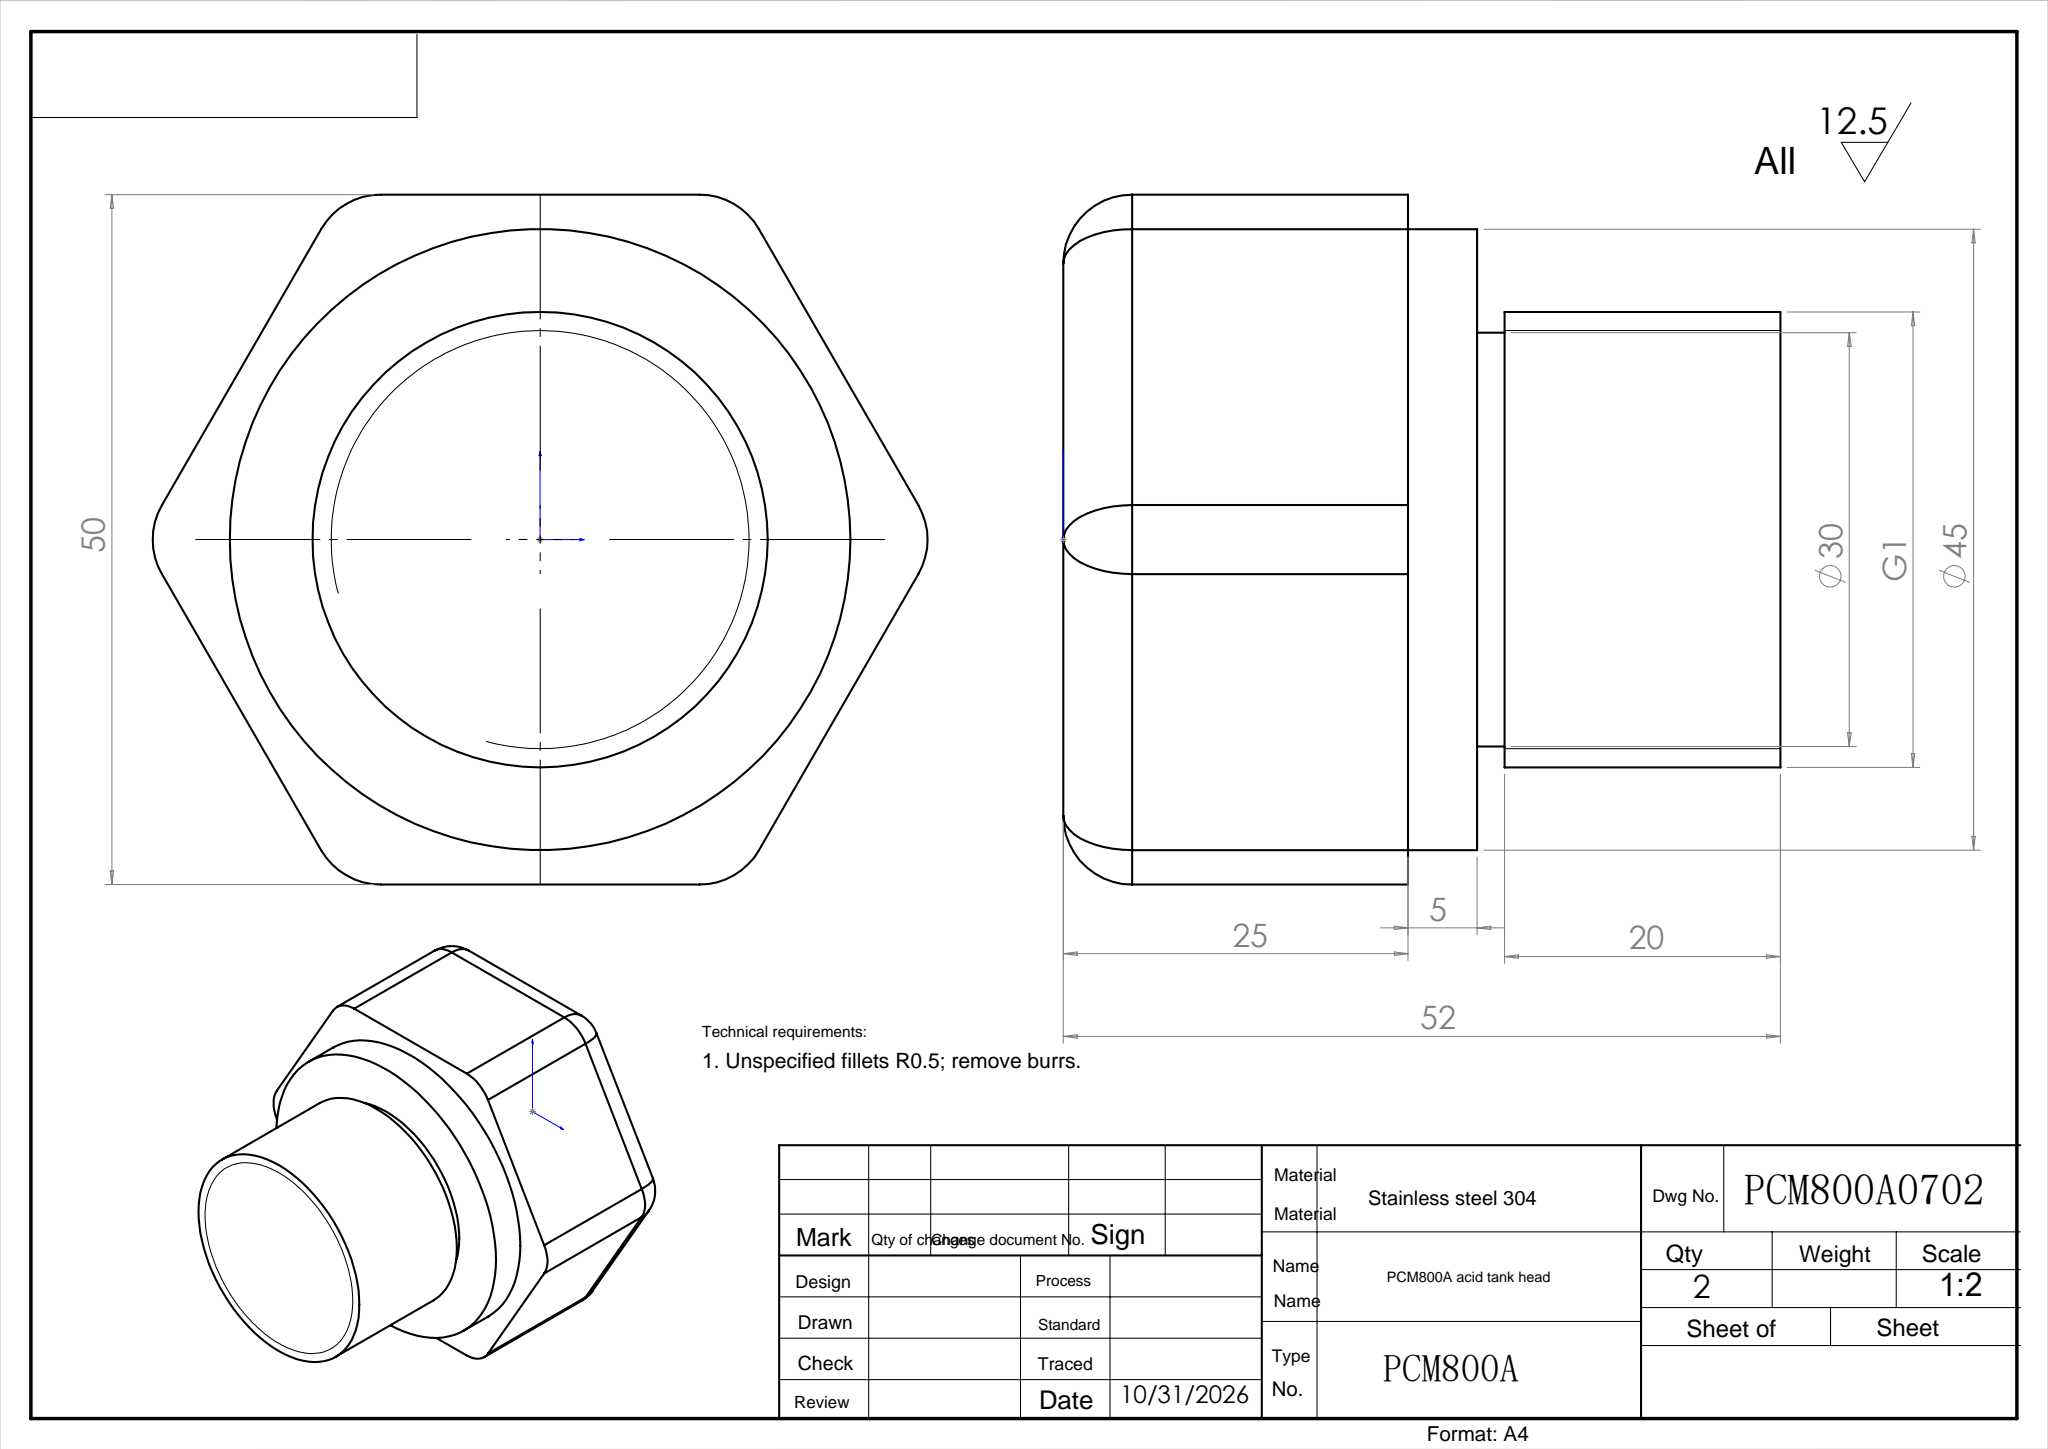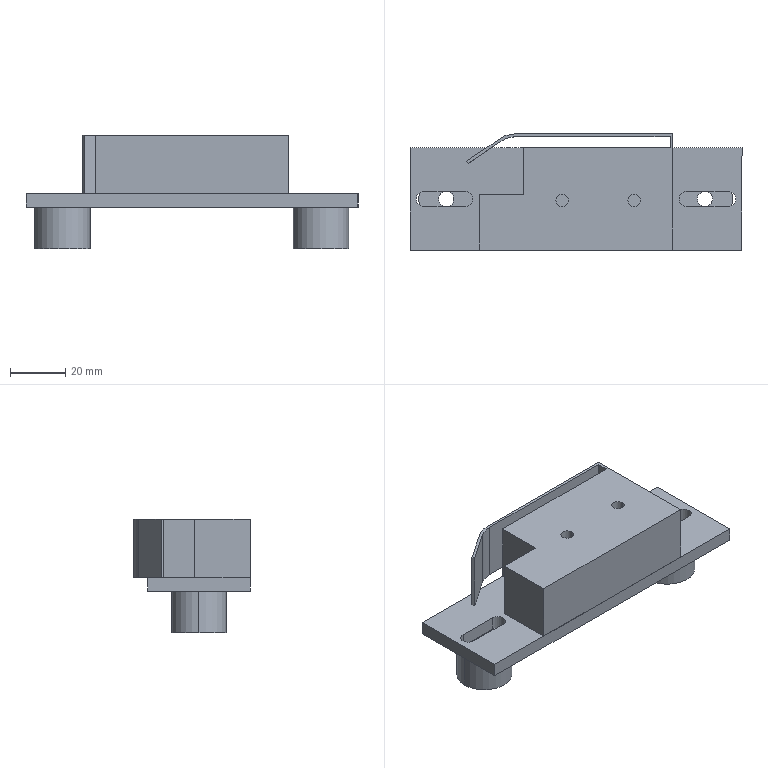Part | SolidWorks | 4 solids | 48 faces | box 120 x 42 x 41 mm | volume 79565 mm3 | plane 28 | cylinder 20 | commonest cylinder face diameters 5.5 x10 20 x6 4.5 x4